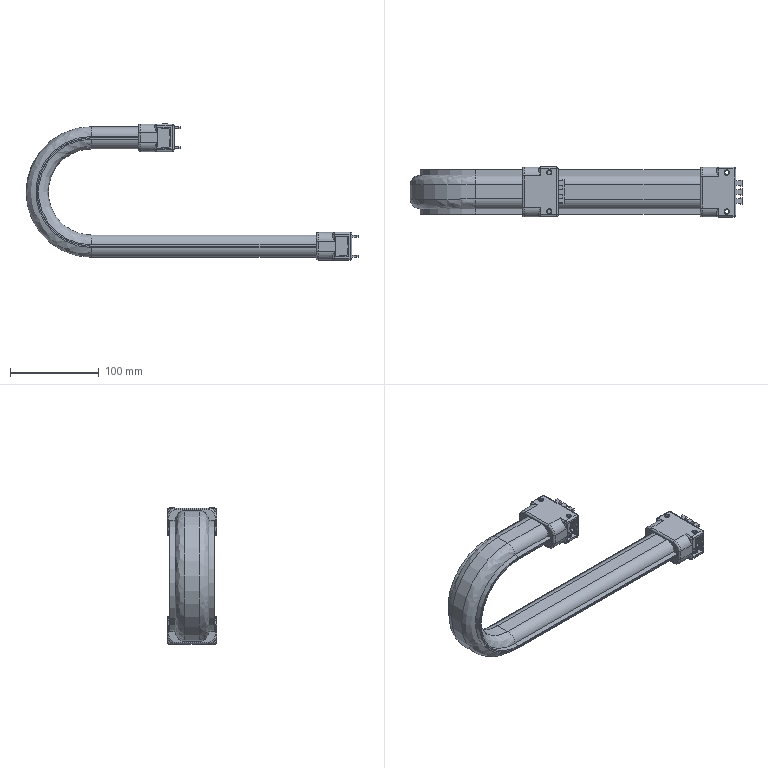Part | SolidWorks | features BaseBody 3 | 3 solids | 511 faces | box 373.5 x 56 x 153.4 mm | volume 213102 mm3 | plane 256 | cylinder 186 | cone 37 | spline 32 | commonest cylinder face diameters 4 x40 4.5 x32 6 x32 7 x32 5 x8 17 x8